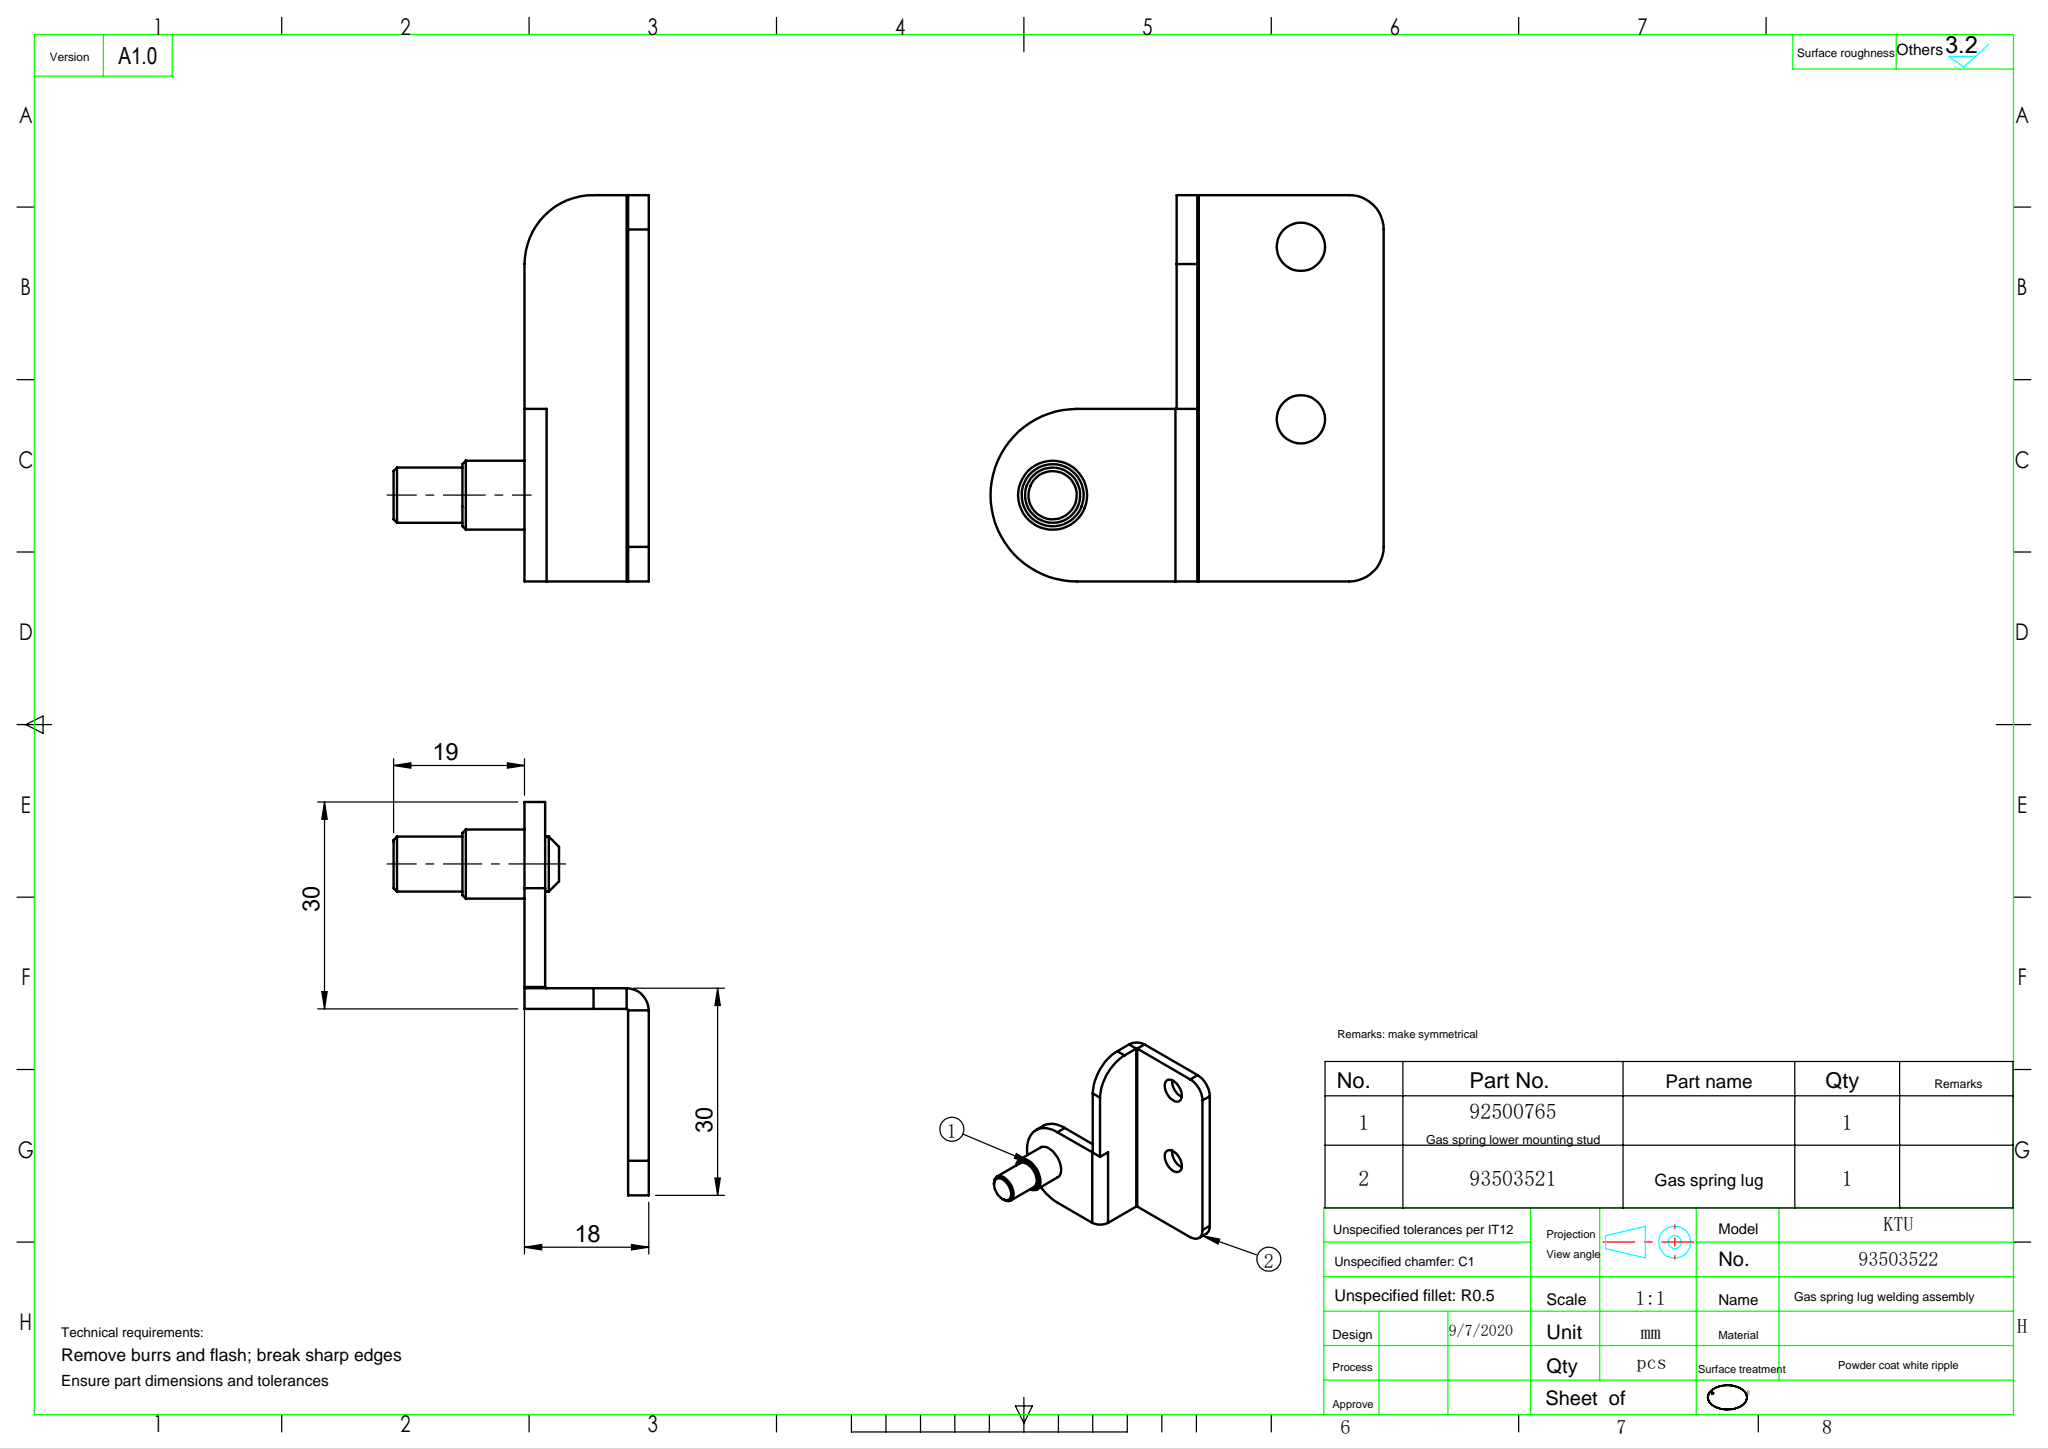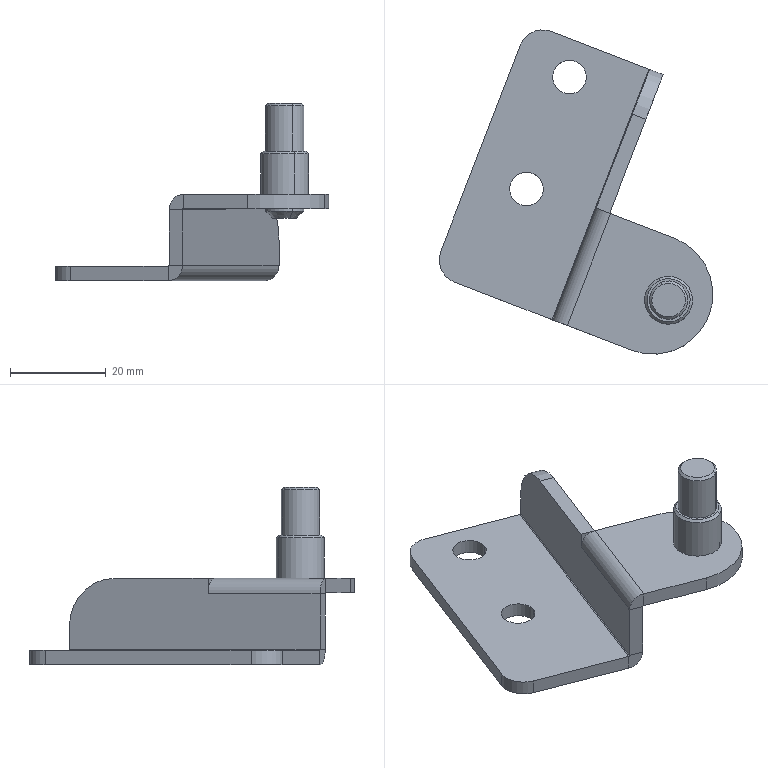Part | SolidWorks | 2 solids | 50 faces | box 57.054 x 67.632 x 37 mm | volume 10154 mm3 | plane 23 | cylinder 21 | cone 6 | commonest cylinder face diameters 7 x4 8 x4 10 x4 0.4 x2 6.4 x2 8.1 x2